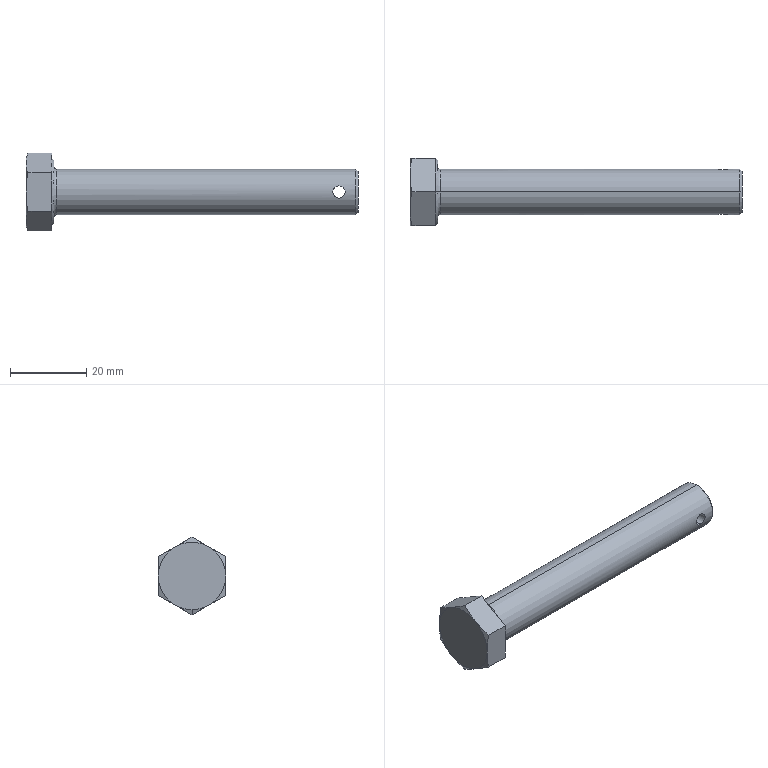Part | SolidWorks | features RevCut 3, Boss 1, Chamfer 1, Cut 1, Extrusion 1, Fillet 1, LPattern 1 | 1 solid | 32 faces | box 87.32 x 17.73 x 20.473 mm | volume 10914 mm3 | plane 15 | cone 11 | cylinder 4 | torus 2 | commonest cylinder face diameters 3.2 x2 12 x2
STEP:
#1=CARTESIAN_POINT('',(7.92,0.,6.));
#2=VERTEX_POINT('',#1);
#3=CARTESIAN_POINT('',(7.92,0.,-6.));
#4=VERTEX_POINT('',#3);
#5=CARTESIAN_POINT('',(7.92,0.,0.));
#6=DIRECTION('',(1.,0.,0.));
#7=DIRECTION('',(0.,0.,-1.));
#8=AXIS2_PLACEMENT_3D('',#5,#6,#7);
#9=CIRCLE('',#8,6.);
#10=EDGE_CURVE('',#2,#4,#9,.T.);
#11=ORIENTED_EDGE('',*,*,#10,.F.);
#12=CARTESIAN_POINT('',(7.32,0.,6.6));
#13=VERTEX_POINT('',#12);
#14=CARTESIAN_POINT('',(7.92,0.,6.6));
#15=DIRECTION('',(0.,1.,0.));
#16=DIRECTION('',(0.,0.,1.));
#17=AXIS2_PLACEMENT_3D('',#14,#15,#16);
#18=CIRCLE('',#17,0.6);
#19=EDGE_CURVE('',#2,#13,#18,.T.);
#20=ORIENTED_EDGE('',*,*,#19,.T.);
#21=CARTESIAN_POINT('',(7.32,0.,-6.6));
#22=VERTEX_POINT('',#21);
#23=CARTESIAN_POINT('',(7.32,0.,0.));
#24=DIRECTION('',(-1.,0.,0.));
#25=DIRECTION('',(0.,0.,-1.));
#26=AXIS2_PLACEMENT_3D('',#23,#24,#25);
#27=CIRCLE('',#26,6.6);
#28=EDGE_CURVE('',#22,#13,#27,.T.);
#29=ORIENTED_EDGE('',*,*,#28,.F.);
#30=CARTESIAN_POINT('',(7.92,0.,-6.6));
#31=DIRECTION('',(0.,-1.,0.));
#32=DIRECTION('',(0.,0.,-1.));
#33=AXIS2_PLACEMENT_3D('',#30,#31,#32);
#34=CIRCLE('',#33,0.6);
#35=EDGE_CURVE('',#4,#22,#34,.T.);
#36=ORIENTED_EDGE('',*,*,#35,.F.);
#37=EDGE_LOOP('',(#11,#20,#29,#36));
#38=FACE_OUTER_BOUND('',#37,.T.);
#39=CARTESIAN_POINT('',(7.92,0.,0.));
#40=DIRECTION('',(1.,0.,0.));
#41=DIRECTION('',(0.,0.,-1.));
#42=AXIS2_PLACEMENT_3D('',#39,#40,#41);
#43=TOROIDAL_SURFACE('',#42,6.6,0.6);
#44=ADVANCED_FACE('',(#38),#43,.F.);
#45=CARTESIAN_POINT('',(82.32,-5.783,-1.6));
#46=VERTEX_POINT('',#45);
#47=CARTESIAN_POINT('',(82.32,-5.783,1.6));
#48=VERTEX_POINT('',#47);
#49=CARTESIAN_POINT('',(82.32,-5.783,-1.6));
#50=CARTESIAN_POINT('',(82.111,-5.783,-1.6));
#51=CARTESIAN_POINT('',(81.899,-5.795,-1.558));
#52=CARTESIAN_POINT('',(81.61,-5.825,-1.438));
#53=CARTESIAN_POINT('',(81.517,-5.838,-1.388));
#54=CARTESIAN_POINT('',(81.343,-5.864,-1.271));
#55=CARTESIAN_POINT('',(81.263,-5.878,-1.206));
#56=CARTESIAN_POINT('',(81.115,-5.906,-1.058));
#57=CARTESIAN_POINT('',(81.048,-5.921,-0.9764));
#58=CARTESIAN_POINT('',(80.933,-5.947,-0.8037));
#59=CARTESIAN_POINT('',(80.883,-5.958,-0.712));
#60=CARTESIAN_POINT('',(80.762,-5.989,-0.4197));
#61=CARTESIAN_POINT('',(80.72,-6.,-0.2114));
#62=CARTESIAN_POINT('',(80.72,-6.,0.1051));
#63=CARTESIAN_POINT('',(80.73,-5.997,0.2093));
#64=CARTESIAN_POINT('',(80.771,-5.987,0.415));
#65=CARTESIAN_POINT('',(80.802,-5.978,0.5171));
#66=CARTESIAN_POINT('',(80.922,-5.949,0.8065));
#67=CARTESIAN_POINT('',(81.041,-5.921,0.9841));
#68=CARTESIAN_POINT('',(81.335,-5.864,1.278));
#69=CARTESIAN_POINT('',(81.512,-5.836,1.397));
#70=CARTESIAN_POINT('',(81.801,-5.805,1.517));
#71=CARTESIAN_POINT('',(81.903,-5.797,1.548));
#72=CARTESIAN_POINT('',(82.109,-5.786,1.59));
#73=CARTESIAN_POINT('',(82.214,-5.783,1.6));
#74=CARTESIAN_POINT('',(82.32,-5.783,1.6));
#75=B_SPLINE_CURVE_WITH_KNOTS('',3,(#49,#50,#51,#52,#53,#54,#55,#56,#57,#58,#59,#60,#61,#62,#63,#64,#65,#66,#67,#68,#69,#70,#71,#72,#73,#74),.UNSPECIFIED.,.F.,.F.,(4,2,2,2,2,2,2,2,2,2,2,2,4),(0.005025,0.005653,0.005967,0.006281,0.006595,0.006909,0.007537,0.007851,0.008165,0.008793,0.009421,0.009735,0.01005),.UNSPECIFIED.);
#76=EDGE_CURVE('',#46,#48,#75,.T.);
#77=ORIENTED_EDGE('',*,*,#76,.F.);
#78=CARTESIAN_POINT('',(82.32,5.783,-1.6));
#79=VERTEX_POINT('',#78);
#80=CARTESIAN_POINT('',(82.32,-8.865,-1.6));
#81=DIRECTION('',(0.,1.,0.));
#82=VECTOR('',#81,1000.);
#83=LINE('',#80,#82);
#84=EDGE_CURVE('',#46,#79,#83,.T.);
#85=ORIENTED_EDGE('',*,*,#84,.T.);
#86=CARTESIAN_POINT('',(82.32,5.783,1.6));
#87=VERTEX_POINT('',#86);
#88=CARTESIAN_POINT('',(82.32,5.783,1.6));
#89=CARTESIAN_POINT('',(82.214,5.783,1.6));
#90=CARTESIAN_POINT('',(82.109,5.786,1.59));
#91=CARTESIAN_POINT('',(81.904,5.797,1.549));
#92=CARTESIAN_POINT('',(81.802,5.805,1.518));
#93=CARTESIAN_POINT('',(81.609,5.826,1.437));
#94=CARTESIAN_POINT('',(81.517,5.838,1.388));
#95=CARTESIAN_POINT('',(81.344,5.864,1.272));
#96=CARTESIAN_POINT('',(81.262,5.878,1.205));
#97=CARTESIAN_POINT('',(81.042,5.921,0.9842));
#98=CARTESIAN_POINT('',(80.922,5.949,0.8065));
#99=CARTESIAN_POINT('',(80.763,5.988,0.4217));
#100=CARTESIAN_POINT('',(80.72,6.,0.2105));
#101=CARTESIAN_POINT('',(80.72,6.,-0.1042));
#102=CARTESIAN_POINT('',(80.73,5.997,-0.2108));
#103=CARTESIAN_POINT('',(80.772,5.986,-0.4164));
#104=CARTESIAN_POINT('',(80.802,5.979,-0.5164));
#105=CARTESIAN_POINT('',(80.923,5.949,-0.808));
#106=CARTESIAN_POINT('',(81.041,5.921,-0.9838));
#107=CARTESIAN_POINT('',(81.263,5.878,-1.206));
#108=CARTESIAN_POINT('',(81.343,5.864,-1.272));
#109=CARTESIAN_POINT('',(81.516,5.838,-1.387));
#110=CARTESIAN_POINT('',(81.61,5.825,-1.438));
#111=CARTESIAN_POINT('',(81.803,5.805,-1.518));
#112=CARTESIAN_POINT('',(81.903,5.797,-1.548));
#113=CARTESIAN_POINT('',(82.109,5.786,-1.59));
#114=CARTESIAN_POINT('',(82.215,5.783,-1.6));
#115=CARTESIAN_POINT('',(82.32,5.783,-1.6));
#116=B_SPLINE_CURVE_WITH_KNOTS('',3,(#88,#89,#90,#91,#92,#93,#94,#95,#96,#97,#98,#99,#100,#101,#102,#103,#104,#105,#106,#107,#108,#109,#110,#111,#112,#113,#114,#115),.UNSPECIFIED.,.F.,.F.,(4,2,2,2,2,2,2,2,2,2,2,2,2,4),(0.,0.0003141,0.0006281,0.0009422,0.001256,0.001884,0.002513,0.002827,0.003141,0.003769,0.004083,0.004397,0.004711,0.005025),.UNSPECIFIED.);
#117=EDGE_CURVE('',#87,#79,#116,.T.);
#118=ORIENTED_EDGE('',*,*,#117,.F.);
#119=CARTESIAN_POINT('',(82.32,-8.865,1.6));
#120=DIRECTION('',(0.,1.,0.));
#121=VECTOR('',#120,1000.);
#122=LINE('',#119,#121);
#123=EDGE_CURVE('',#48,#87,#122,.T.);
#124=ORIENTED_EDGE('',*,*,#123,.F.);
#125=EDGE_LOOP('',(#77,#85,#118,#124));
#126=FACE_OUTER_BOUND('',#125,.T.);
#127=CARTESIAN_POINT('',(82.32,-8.865,0.));
#128=DIRECTION('',(0.,1.,0.));
#129=DIRECTION('',(0.,0.,1.));
#130=AXIS2_PLACEMENT_3D('',#127,#128,#129);
#131=CYLINDRICAL_SURFACE('',#130,1.6);
#132=ADVANCED_FACE('',(#126),#131,.F.);
#133=CARTESIAN_POINT('',(87.32,0.,-5.4));
#134=VERTEX_POINT('',#133);
#135=CARTESIAN_POINT('',(87.32,0.,5.4));
#136=VERTEX_POINT('',#135);
#137=CARTESIAN_POINT('',(87.32,0.,0.));
#138=DIRECTION('',(1.,0.,0.));
#139=DIRECTION('',(0.,0.,-1.));
#140=AXIS2_PLACEMENT_3D('',#137,#138,#139);
#141=CIRCLE('',#140,5.4);
#142=EDGE_CURVE('',#134,#136,#141,.T.);
#143=ORIENTED_EDGE('',*,*,#142,.F.);
#144=CARTESIAN_POINT('',(86.72,0.,-6.));
#145=VERTEX_POINT('',#144);
#146=CARTESIAN_POINT('',(87.32,0.,-5.4));
#147=DIRECTION('',(-0.7071,0.,-0.7071));
#148=VECTOR('',#147,1000.);
#149=LINE('',#146,#148);
#150=EDGE_CURVE('',#134,#145,#149,.T.);
#151=ORIENTED_EDGE('',*,*,#150,.T.);
#152=CARTESIAN_POINT('',(86.72,0.,6.));
#153=VERTEX_POINT('',#152);
#154=CARTESIAN_POINT('',(86.72,0.,0.));
#155=DIRECTION('',(-1.,0.,0.));
#156=DIRECTION('',(0.,0.,-1.));
#157=AXIS2_PLACEMENT_3D('',#154,#155,#156);
#158=CIRCLE('',#157,6.);
#159=EDGE_CURVE('',#153,#145,#158,.T.);
#160=ORIENTED_EDGE('',*,*,#159,.F.);
#161=CARTESIAN_POINT('',(87.32,0.,5.4));
#162=DIRECTION('',(-0.7071,0.,0.7071));
#163=VECTOR('',#162,1000.);
#164=LINE('',#161,#163);
#165=EDGE_CURVE('',#136,#153,#164,.T.);
#166=ORIENTED_EDGE('',*,*,#165,.F.);
#167=EDGE_LOOP('',(#143,#151,#160,#166));
#168=FACE_OUTER_BOUND('',#167,.T.);
#169=CARTESIAN_POINT('',(87.32,0.,0.));
#170=DIRECTION('',(-1.,0.,0.));
#171=DIRECTION('',(0.,0.,1.));
#172=AXIS2_PLACEMENT_3D('',#169,#170,#171);
#173=CONICAL_SURFACE('',#172,5.4,0.7854);
#174=ADVANCED_FACE('',(#168),#173,.T.);
#175=ORIENTED_EDGE('',*,*,#117,.T.);
#176=CARTESIAN_POINT('',(82.32,5.783,-1.6));
#177=CARTESIAN_POINT('',(82.529,5.783,-1.6));
#178=CARTESIAN_POINT('',(82.741,5.795,-1.558));
#179=CARTESIAN_POINT('',(83.03,5.825,-1.438));
#180=CARTESIAN_POINT('',(83.123,5.838,-1.388));
#181=CARTESIAN_POINT('',(83.297,5.864,-1.271));
#182=CARTESIAN_POINT('',(83.377,5.878,-1.206));
#183=CARTESIAN_POINT('',(83.525,5.906,-1.058));
#184=CARTESIAN_POINT('',(83.592,5.921,-0.9764));
#185=CARTESIAN_POINT('',(83.707,5.947,-0.8037));
#186=CARTESIAN_POINT('',(83.757,5.958,-0.712));
#187=CARTESIAN_POINT('',(83.878,5.989,-0.4197));
#188=CARTESIAN_POINT('',(83.92,6.,-0.2114));
#189=CARTESIAN_POINT('',(83.92,6.,0.1051));
#190=CARTESIAN_POINT('',(83.91,5.997,0.2093));
#191=CARTESIAN_POINT('',(83.869,5.987,0.415));
#192=CARTESIAN_POINT('',(83.838,5.978,0.5171));
#193=CARTESIAN_POINT('',(83.718,5.949,0.8065));
#194=CARTESIAN_POINT('',(83.599,5.921,0.9841));
#195=CARTESIAN_POINT('',(83.305,5.864,1.278));
#196=CARTESIAN_POINT('',(83.128,5.836,1.397));
#197=CARTESIAN_POINT('',(82.839,5.805,1.517));
#198=CARTESIAN_POINT('',(82.737,5.797,1.548));
#199=CARTESIAN_POINT('',(82.531,5.786,1.59));
#200=CARTESIAN_POINT('',(82.426,5.783,1.6));
#201=CARTESIAN_POINT('',(82.32,5.783,1.6));
#202=B_SPLINE_CURVE_WITH_KNOTS('',3,(#176,#177,#178,#179,#180,#181,#182,#183,#184,#185,#186,#187,#188,#189,#190,#191,#192,#193,#194,#195,#196,#197,#198,#199,#200,#201),.UNSPECIFIED.,.F.,.F.,(4,2,2,2,2,2,2,2,2,2,2,2,4),(0.005025,0.005653,0.005967,0.006281,0.006595,0.006909,0.007537,0.007851,0.008165,0.008793,0.009421,0.009735,0.01005),.UNSPECIFIED.);
#203=EDGE_CURVE('',#79,#87,#202,.T.);
#204=ORIENTED_EDGE('',*,*,#203,.T.);
#205=EDGE_LOOP('',(#175,#204));
#206=FACE_BOUND('',#205,.T.);
#207=ORIENTED_EDGE('',*,*,#159,.T.);
#208=CARTESIAN_POINT('',(87.32,0.,-6.));
#209=DIRECTION('',(-1.,0.,0.));
#210=VECTOR('',#209,1000.);
#211=LINE('',#208,#210);
#212=EDGE_CURVE('',#145,#4,#211,.T.);
#213=ORIENTED_EDGE('',*,*,#212,.T.);
#214=CARTESIAN_POINT('',(7.92,0.,0.));
#215=DIRECTION('',(1.,0.,0.));
#216=DIRECTION('',(0.,0.,-1.));
#217=AXIS2_PLACEMENT_3D('',#214,#215,#216);
#218=CIRCLE('',#217,6.);
#219=EDGE_CURVE('',#4,#2,#218,.T.);
#220=ORIENTED_EDGE('',*,*,#219,.T.);
#221=CARTESIAN_POINT('',(87.32,0.,6.));
#222=DIRECTION('',(-1.,0.,0.));
#223=VECTOR('',#222,1000.);
#224=LINE('',#221,#223);
#225=EDGE_CURVE('',#153,#2,#224,.T.);
#226=ORIENTED_EDGE('',*,*,#225,.F.);
#227=EDGE_LOOP('',(#207,#213,#220,#226));
#228=FACE_OUTER_BOUND('',#227,.T.);
#229=CARTESIAN_POINT('',(87.32,0.,0.));
#230=DIRECTION('',(-1.,0.,0.));
#231=DIRECTION('',(0.,0.,1.));
#232=AXIS2_PLACEMENT_3D('',#229,#230,#231);
#233=CYLINDRICAL_SURFACE('',#232,6.);
#234=ADVANCED_FACE('',(#206,#228),#233,.T.);
#235=CARTESIAN_POINT('',(0.,-4.432,-7.677));
#236=VERTEX_POINT('',#235);
#237=CARTESIAN_POINT('',(0.,0.,-8.865));
#238=VERTEX_POINT('',#237);
#239=CARTESIAN_POINT('',(0.,0.,0.));
#240=DIRECTION('',(1.,0.,0.));
#241=DIRECTION('',(0.,0.,-1.));
#242=AXIS2_PLACEMENT_3D('',#239,#240,#241);
#243=CIRCLE('',#242,8.865);
#244=EDGE_CURVE('',#236,#238,#243,.T.);
#245=ORIENTED_EDGE('',*,*,#244,.T.);
#246=CARTESIAN_POINT('',(0.4992,0.,-10.236));
#247=VERTEX_POINT('',#246);
#248=CARTESIAN_POINT('',(0.,0.,-8.865));
#249=DIRECTION('',(0.342,0.,-0.9397));
#250=VECTOR('',#249,1000.);
#251=LINE('',#248,#250);
#252=EDGE_CURVE('',#238,#247,#251,.T.);
#253=ORIENTED_EDGE('',*,*,#252,.T.);
#254=CARTESIAN_POINT('',(0.4992,0.,-10.236));
#255=CARTESIAN_POINT('',(0.3439,-0.7387,-9.81));
#256=CARTESIAN_POINT('',(0.2179,-1.477,-9.383));
#257=CARTESIAN_POINT('',(0.04564,-2.955,-8.53));
#258=CARTESIAN_POINT('',(0.,-3.694,-8.104));
#259=CARTESIAN_POINT('',(0.,-4.432,-7.677));
#260=B_SPLINE_CURVE_WITH_KNOTS('',3,(#254,#255,#256,#257,#258,#259),.UNSPECIFIED.,.F.,.F.,(4,2,4),(0.000000231,0.002559,0.005118),.UNSPECIFIED.);
#261=EDGE_CURVE('',#247,#236,#260,.T.);
#262=ORIENTED_EDGE('',*,*,#261,.T.);
#263=EDGE_LOOP('',(#245,#253,#262));
#264=FACE_OUTER_BOUND('',#263,.T.);
#265=CARTESIAN_POINT('',(0.,0.,0.));
#266=DIRECTION('',(1.,0.,0.));
#267=DIRECTION('',(0.,0.,-1.));
#268=AXIS2_PLACEMENT_3D('',#265,#266,#267);
#269=CONICAL_SURFACE('',#268,8.865,1.222);
#270=ADVANCED_FACE('',(#264),#269,.T.);
#271=CARTESIAN_POINT('',(7.32,0.,8.315));
#272=VERTEX_POINT('',#271);
#273=CARTESIAN_POINT('',(7.32,0.,-8.315));
#274=VERTEX_POINT('',#273);
#275=CARTESIAN_POINT('',(7.32,0.,0.));
#276=DIRECTION('',(-1.,0.,0.));
#277=DIRECTION('',(0.,0.,1.));
#278=AXIS2_PLACEMENT_3D('',#275,#276,#277);
#279=CIRCLE('',#278,8.315);
#280=EDGE_CURVE('',#272,#274,#279,.T.);
#281=ORIENTED_EDGE('',*,*,#280,.T.);
#282=CARTESIAN_POINT('',(6.72,0.,-8.915));
#283=VERTEX_POINT('',#282);
#284=CARTESIAN_POINT('',(6.72,0.,-8.915));
#285=DIRECTION('',(-0.7071,0.,-0.7071));
#286=VECTOR('',#285,1000.);
#287=LINE('',#284,#286);
#288=EDGE_CURVE('',#274,#283,#287,.T.);
#289=ORIENTED_EDGE('',*,*,#288,.T.);
#290=CARTESIAN_POINT('',(6.72,3.616,-8.149));
#291=VERTEX_POINT('',#290);
#292=CARTESIAN_POINT('',(6.72,0.,0.));
#293=DIRECTION('',(-1.,0.,0.));
#294=DIRECTION('',(0.,0.,1.));
#295=AXIS2_PLACEMENT_3D('',#292,#293,#294);
#296=CIRCLE('',#295,8.915);
#297=EDGE_CURVE('',#291,#283,#296,.T.);
#298=ORIENTED_EDGE('',*,*,#297,.F.);
#299=CARTESIAN_POINT('',(6.72,5.249,-7.206));
#300=VERTEX_POINT('',#299);
#301=CARTESIAN_POINT('',(6.72,3.616,-8.149));
#302=CARTESIAN_POINT('',(6.786,4.16,-7.834));
#303=CARTESIAN_POINT('',(6.786,4.705,-7.52));
#304=CARTESIAN_POINT('',(6.72,5.249,-7.206));
#305=B_SPLINE_CURVE_WITH_KNOTS('',3,(#301,#302,#303,#304),.UNSPECIFIED.,.F.,.F.,(4,4),(0.000001889,0.001888),.UNSPECIFIED.);
#306=EDGE_CURVE('',#291,#300,#305,.T.);
#307=ORIENTED_EDGE('',*,*,#306,.T.);
#308=CARTESIAN_POINT('',(6.72,8.865,-0.9429));
#309=VERTEX_POINT('',#308);
#310=CARTESIAN_POINT('',(6.72,0.,0.));
#311=DIRECTION('',(-1.,0.,0.));
#312=DIRECTION('',(0.,0.,1.));
#313=AXIS2_PLACEMENT_3D('',#310,#311,#312);
#314=CIRCLE('',#313,8.915);
#315=EDGE_CURVE('',#309,#300,#314,.T.);
#316=ORIENTED_EDGE('',*,*,#315,.F.);
#317=CARTESIAN_POINT('',(6.72,8.865,0.9429));
#318=VERTEX_POINT('',#317);
#319=CARTESIAN_POINT('',(6.72,8.865,-0.9429));
#320=CARTESIAN_POINT('',(6.787,8.865,-0.3136));
#321=CARTESIAN_POINT('',(6.786,8.865,0.315));
#322=CARTESIAN_POINT('',(6.72,8.865,0.9429));
#323=B_SPLINE_CURVE_WITH_KNOTS('',3,(#319,#320,#321,#322),.UNSPECIFIED.,.F.,.F.,(4,4),(0.004033,0.005912),.UNSPECIFIED.);
#324=EDGE_CURVE('',#309,#318,#323,.T.);
#325=ORIENTED_EDGE('',*,*,#324,.T.);
#326=CARTESIAN_POINT('',(6.72,5.249,7.206));
#327=VERTEX_POINT('',#326);
#328=CARTESIAN_POINT('',(6.72,0.,0.));
#329=DIRECTION('',(-1.,0.,0.));
#330=DIRECTION('',(0.,0.,1.));
#331=AXIS2_PLACEMENT_3D('',#328,#329,#330);
#332=CIRCLE('',#331,8.915);
#333=EDGE_CURVE('',#327,#318,#332,.T.);
#334=ORIENTED_EDGE('',*,*,#333,.F.);
#335=CARTESIAN_POINT('',(6.72,3.616,8.149));
#336=VERTEX_POINT('',#335);
#337=CARTESIAN_POINT('',(6.72,5.249,7.206));
#338=CARTESIAN_POINT('',(6.786,4.705,7.52));
#339=CARTESIAN_POINT('',(6.786,4.16,7.834));
#340=CARTESIAN_POINT('',(6.72,3.616,8.149));
#341=B_SPLINE_CURVE_WITH_KNOTS('',3,(#337,#338,#339,#340),.UNSPECIFIED.,.F.,.F.,(4,4),(0.000001889,0.001888),.UNSPECIFIED.);
#342=EDGE_CURVE('',#327,#336,#341,.T.);
#343=ORIENTED_EDGE('',*,*,#342,.T.);
#344=CARTESIAN_POINT('',(6.72,0.,8.915));
#345=VERTEX_POINT('',#344);
#346=CARTESIAN_POINT('',(6.72,0.,0.));
#347=DIRECTION('',(-1.,0.,0.));
#348=DIRECTION('',(0.,0.,1.));
#349=AXIS2_PLACEMENT_3D('',#346,#347,#348);
#350=CIRCLE('',#349,8.915);
#351=EDGE_CURVE('',#345,#336,#350,.T.);
#352=ORIENTED_EDGE('',*,*,#351,.F.);
#353=CARTESIAN_POINT('',(6.72,0.,8.915));
#354=DIRECTION('',(-0.7071,0.,0.7071));
#355=VECTOR('',#354,1000.);
#356=LINE('',#353,#355);
#357=EDGE_CURVE('',#272,#345,#356,.T.);
#358=ORIENTED_EDGE('',*,*,#357,.F.);
#359=EDGE_LOOP('',(#281,#289,#298,#307,#316,#325,#334,#343,#352,#358));
#360=FACE_OUTER_BOUND('',#359,.T.);
#361=CARTESIAN_POINT('',(6.72,0.,0.));
#362=DIRECTION('',(-1.,0.,0.));
#363=DIRECTION('',(0.,0.,1.));
#364=AXIS2_PLACEMENT_3D('',#361,#362,#363);
#365=CONICAL_SURFACE('',#364,8.915,0.7854);
#366=ADVANCED_FACE('',(#360),#365,.T.);
#367=ORIENTED_EDGE('',*,*,#28,.T.);
#368=CARTESIAN_POINT('',(7.32,0.,0.));
#369=DIRECTION('',(-1.,0.,0.));
#370=DIRECTION('',(0.,0.,-1.));
#371=AXIS2_PLACEMENT_3D('',#368,#369,#370);
#372=CIRCLE('',#371,6.6);
#373=EDGE_CURVE('',#13,#22,#372,.T.);
#374=ORIENTED_EDGE('',*,*,#373,.T.);
#375=EDGE_LOOP('',(#367,#374));
#376=FACE_BOUND('',#375,.T.);
#377=ORIENTED_EDGE('',*,*,#280,.F.);
#378=CARTESIAN_POINT('',(7.32,0.,0.));
#379=DIRECTION('',(-1.,0.,0.));
#380=DIRECTION('',(0.,0.,1.));
#381=AXIS2_PLACEMENT_3D('',#378,#379,#380);
#382=CIRCLE('',#381,8.315);
#383=EDGE_CURVE('',#274,#272,#382,.T.);
#384=ORIENTED_EDGE('',*,*,#383,.F.);
#385=EDGE_LOOP('',(#377,#384));
#386=FACE_OUTER_BOUND('',#385,.T.);
#387=CARTESIAN_POINT('',(7.32,0.,-10.236));
#388=DIRECTION('',(1.,0.,0.));
#389=DIRECTION('',(0.,0.,-1.));
#390=AXIS2_PLACEMENT_3D('',#387,#388,#389);
#391=PLANE('',#390);
#392=ADVANCED_FACE('',(#376,#386),#391,.T.);
#393=ORIENTED_EDGE('',*,*,#261,.F.);
#394=CARTESIAN_POINT('',(6.72,0.,-10.236));
#395=VERTEX_POINT('',#394);
#396=CARTESIAN_POINT('',(7.32,0.,-10.236));
#397=DIRECTION('',(-1.,0.,0.));
#398=VECTOR('',#397,1000.);
#399=LINE('',#396,#398);
#400=EDGE_CURVE('',#395,#247,#399,.T.);
#401=ORIENTED_EDGE('',*,*,#400,.F.);
#402=CARTESIAN_POINT('',(6.72,-3.616,-8.149));
#403=VERTEX_POINT('',#402);
#404=CARTESIAN_POINT('',(6.72,-8.865,-5.118));
#405=DIRECTION('',(0.,0.866,-0.5));
#406=VECTOR('',#405,1000.);
#407=LINE('',#404,#406);
#408=EDGE_CURVE('',#403,#395,#407,.T.);
#409=ORIENTED_EDGE('',*,*,#408,.F.);
#410=CARTESIAN_POINT('',(6.72,-5.249,-7.206));
#411=VERTEX_POINT('',#410);
#412=CARTESIAN_POINT('',(6.72,-5.249,-7.206));
#413=CARTESIAN_POINT('',(6.786,-4.705,-7.52));
#414=CARTESIAN_POINT('',(6.786,-4.16,-7.834));
#415=CARTESIAN_POINT('',(6.72,-3.616,-8.149));
#416=B_SPLINE_CURVE_WITH_KNOTS('',3,(#412,#413,#414,#415),.UNSPECIFIED.,.F.,.F.,(4,4),(0.000001889,0.001888),.UNSPECIFIED.);
#417=EDGE_CURVE('',#411,#403,#416,.T.);
#418=ORIENTED_EDGE('',*,*,#417,.F.);
#419=CARTESIAN_POINT('',(6.72,-8.865,-5.118));
#420=VERTEX_POINT('',#419);
#421=CARTESIAN_POINT('',(6.72,-8.865,-5.118));
#422=DIRECTION('',(0.,0.866,-0.5));
#423=VECTOR('',#422,1000.);
#424=LINE('',#421,#423);
#425=EDGE_CURVE('',#420,#411,#424,.T.);
#426=ORIENTED_EDGE('',*,*,#425,.F.);
#427=CARTESIAN_POINT('',(0.4992,-8.865,-5.118));
#428=VERTEX_POINT('',#427);
#429=CARTESIAN_POINT('',(7.32,-8.865,-5.118));
#430=DIRECTION('',(-1.,0.,0.));
#431=VECTOR('',#430,1000.);
#432=LINE('',#429,#431);
#433=EDGE_CURVE('',#420,#428,#432,.T.);
#434=ORIENTED_EDGE('',*,*,#433,.T.);
#435=CARTESIAN_POINT('',(0.,-4.432,-7.677));
#436=CARTESIAN_POINT('',(0.,-5.171,-7.251));
#437=CARTESIAN_POINT('',(0.04564,-5.91,-6.824));
#438=CARTESIAN_POINT('',(0.2179,-7.387,-5.971));
#439=CARTESIAN_POINT('',(0.3439,-8.126,-5.545));
#440=CARTESIAN_POINT('',(0.4992,-8.865,-5.118));
#441=B_SPLINE_CURVE_WITH_KNOTS('',3,(#435,#436,#437,#438,#439,#440),.UNSPECIFIED.,.F.,.F.,(4,2,4),(0.005118,0.007678,0.01024),.UNSPECIFIED.);
#442=EDGE_CURVE('',#236,#428,#441,.T.);
#443=ORIENTED_EDGE('',*,*,#442,.F.);
#444=EDGE_LOOP('',(#393,#401,#409,#418,#426,#434,#443));
#445=FACE_OUTER_BOUND('',#444,.T.);
#446=CARTESIAN_POINT('',(7.32,-8.865,-5.118));
#447=DIRECTION('',(0.,0.5,0.866));
#448=DIRECTION('',(0.,-0.866,0.5));
#449=AXIS2_PLACEMENT_3D('',#446,#447,#448);
#450=PLANE('',#449);
#451=ADVANCED_FACE('',(#445),#450,.F.);
#452=CARTESIAN_POINT('',(0.4992,8.865,-5.118));
#453=VERTEX_POINT('',#452);
#454=CARTESIAN_POINT('',(0.,4.433,-7.677));
#455=VERTEX_POINT('',#454);
#456=CARTESIAN_POINT('',(0.4992,8.865,-5.118));
#457=CARTESIAN_POINT('',(0.3439,8.126,-5.545));
#458=CARTESIAN_POINT('',(0.2179,7.388,-5.971));
#459=CARTESIAN_POINT('',(0.04564,5.91,-6.824));
#460=CARTESIAN_POINT('',(0.,5.171,-7.251));
#461=CARTESIAN_POINT('',(0.,4.433,-7.677));
#462=B_SPLINE_CURVE_WITH_KNOTS('',3,(#456,#457,#458,#459,#460,#461),.UNSPECIFIED.,.F.,.F.,(4,2,4),(0.000000231,0.002559,0.005118),.UNSPECIFIED.);
#463=EDGE_CURVE('',#453,#455,#462,.T.);
#464=ORIENTED_EDGE('',*,*,#463,.F.);
#465=CARTESIAN_POINT('',(6.72,8.865,-5.118));
#466=VERTEX_POINT('',#465);
#467=CARTESIAN_POINT('',(7.32,8.865,-5.118));
#468=DIRECTION('',(-1.,0.,0.));
#469=VECTOR('',#468,1000.);
#470=LINE('',#467,#469);
#471=EDGE_CURVE('',#466,#453,#470,.T.);
#472=ORIENTED_EDGE('',*,*,#471,.F.);
#473=CARTESIAN_POINT('',(6.72,0.,-10.236));
#474=DIRECTION('',(0.,0.866,0.5));
#475=VECTOR('',#474,1000.);
#476=LINE('',#473,#475);
#477=EDGE_CURVE('',#300,#466,#476,.T.);
#478=ORIENTED_EDGE('',*,*,#477,.F.);
#479=ORIENTED_EDGE('',*,*,#306,.F.);
#480=CARTESIAN_POINT('',(6.72,0.,-10.236));
#481=DIRECTION('',(0.,0.866,0.5));
#482=VECTOR('',#481,1000.);
#483=LINE('',#480,#482);
#484=EDGE_CURVE('',#395,#291,#483,.T.);
#485=ORIENTED_EDGE('',*,*,#484,.F.);
#486=ORIENTED_EDGE('',*,*,#400,.T.);
#487=CARTESIAN_POINT('',(0.,4.433,-7.677));
#488=CARTESIAN_POINT('',(0.,3.694,-8.104));
#489=CARTESIAN_POINT('',(0.04564,2.955,-8.53));
#490=CARTESIAN_POINT('',(0.2179,1.478,-9.383));
#491=CARTESIAN_POINT('',(0.3439,0.7388,-9.81));
#492=CARTESIAN_POINT('',(0.4992,0.,-10.236));
#493=B_SPLINE_CURVE_WITH_KNOTS('',3,(#487,#488,#489,#490,#491,#492),.UNSPECIFIED.,.F.,.F.,(4,2,4),(0.005118,0.007678,0.01024),.UNSPECIFIED.);
#494=EDGE_CURVE('',#455,#247,#493,.T.);
#495=ORIENTED_EDGE('',*,*,#494,.F.);
#496=EDGE_LOOP('',(#464,#472,#478,#479,#485,#486,#495));
#497=FACE_OUTER_BOUND('',#496,.T.);
#498=CARTESIAN_POINT('',(7.32,0.,-10.236));
#499=DIRECTION('',(0.,-0.5,0.866));
#500=DIRECTION('',(0.,-0.866,-0.5));
#501=AXIS2_PLACEMENT_3D('',#498,#499,#500);
#502=PLANE('',#501);
#503=ADVANCED_FACE('',(#497),#502,.F.);
#504=CARTESIAN_POINT('',(0.4992,8.865,5.118));
#505=VERTEX_POINT('',#504);
#506=CARTESIAN_POINT('',(0.,8.865,0.));
#507=VERTEX_POINT('',#506);
#508=CARTESIAN_POINT('',(0.4992,8.865,5.118));
#509=CARTESIAN_POINT('',(0.3443,8.865,4.267));
#510=CARTESIAN_POINT('',(0.2182,8.865,3.415));
#511=CARTESIAN_POINT('',(0.04582,8.865,1.709));
#512=CARTESIAN_POINT('',(0.,8.865,0.8548));
#513=CARTESIAN_POINT('',(0.,8.865,0.));
#514=B_SPLINE_CURVE_WITH_KNOTS('',3,(#508,#509,#510,#511,#512,#513),.UNSPECIFIED.,.F.,.F.,(4,2,4),(0.01846,0.02104,0.02362),.UNSPECIFIED.);
#515=EDGE_CURVE('',#505,#507,#514,.T.);
#516=ORIENTED_EDGE('',*,*,#515,.F.);
#517=CARTESIAN_POINT('',(6.72,8.865,5.118));
#518=VERTEX_POINT('',#517);
#519=CARTESIAN_POINT('',(7.32,8.865,5.118));
#520=DIRECTION('',(-1.,0.,0.));
#521=VECTOR('',#520,1000.);
#522=LINE('',#519,#521);
#523=EDGE_CURVE('',#518,#505,#522,.T.);
#524=ORIENTED_EDGE('',*,*,#523,.F.);
#525=CARTESIAN_POINT('',(6.72,8.865,-5.118));
#526=DIRECTION('',(0.,0.,1.));
#527=VECTOR('',#526,1000.);
#528=LINE('',#525,#527);
#529=EDGE_CURVE('',#318,#518,#528,.T.);
#530=ORIENTED_EDGE('',*,*,#529,.F.);
#531=ORIENTED_EDGE('',*,*,#324,.F.);
#532=CARTESIAN_POINT('',(6.72,8.865,-5.118));
#533=DIRECTION('',(0.,0.,1.));
#534=VECTOR('',#533,1000.);
#535=LINE('',#532,#534);
#536=EDGE_CURVE('',#466,#309,#535,.T.);
#537=ORIENTED_EDGE('',*,*,#536,.F.);
#538=ORIENTED_EDGE('',*,*,#471,.T.);
#539=CARTESIAN_POINT('',(0.,8.865,0.));
#540=CARTESIAN_POINT('',(0.,8.865,-0.8523));
#541=CARTESIAN_POINT('',(0.04558,8.865,-1.706));
#542=CARTESIAN_POINT('',(0.2181,8.865,-3.414));
#543=CARTESIAN_POINT('',(0.3449,8.865,-4.271));
#544=CARTESIAN_POINT('',(0.4992,8.865,-5.118));
#545=B_SPLINE_CURVE_WITH_KNOTS('',3,(#539,#540,#541,#542,#543,#544),.UNSPECIFIED.,.F.,.F.,(4,2,4),(0.02362,0.02619,0.02876),.UNSPECIFIED.);
#546=EDGE_CURVE('',#507,#453,#545,.T.);
#547=ORIENTED_EDGE('',*,*,#546,.F.);
#548=EDGE_LOOP('',(#516,#524,#530,#531,#537,#538,#547));
#549=FACE_OUTER_BOUND('',#548,.T.);
#550=CARTESIAN_POINT('',(7.32,8.865,-5.118));
#551=DIRECTION('',(0.,-1.,0.));
#552=DIRECTION('',(0.,0.,-1.));
#553=AXIS2_PLACEMENT_3D('',#550,#551,#552);
#554=PLANE('',#553);
#555=ADVANCED_FACE('',(#549),#554,.F.);
#556=CARTESIAN_POINT('',(0.4992,0.,10.236));
#557=VERTEX_POINT('',#556);
#558=CARTESIAN_POINT('',(0.,4.432,7.677));
#559=VERTEX_POINT('',#558);
#560=CARTESIAN_POINT('',(0.4992,0.,10.236));
#561=CARTESIAN_POINT('',(0.3439,0.7387,9.81));
#562=CARTESIAN_POINT('',(0.2179,1.477,9.383));
#563=CARTESIAN_POINT('',(0.04564,2.955,8.53));
#564=CARTESIAN_POINT('',(0.,3.694,8.104));
#565=CARTESIAN_POINT('',(0.,4.432,7.677));
#566=B_SPLINE_CURVE_WITH_KNOTS('',3,(#560,#561,#562,#563,#564,#565),.UNSPECIFIED.,.F.,.F.,(4,2,4),(0.000000231,0.002559,0.005118),.UNSPECIFIED.);
#567=EDGE_CURVE('',#557,#559,#566,.T.);
#568=ORIENTED_EDGE('',*,*,#567,.F.);
#569=CARTESIAN_POINT('',(6.72,0.,10.236));
#570=VERTEX_POINT('',#569);
#571=CARTESIAN_POINT('',(7.32,0.,10.236));
#572=DIRECTION('',(-1.,0.,0.));
#573=VECTOR('',#572,1000.);
#574=LINE('',#571,#573);
#575=EDGE_CURVE('',#570,#557,#574,.T.);
#576=ORIENTED_EDGE('',*,*,#575,.F.);
#577=CARTESIAN_POINT('',(6.72,8.865,5.118));
#578=DIRECTION('',(0.,-0.866,0.5));
#579=VECTOR('',#578,1000.);
#580=LINE('',#577,#579);
#581=EDGE_CURVE('',#336,#570,#580,.T.);
#582=ORIENTED_EDGE('',*,*,#581,.F.);
#583=ORIENTED_EDGE('',*,*,#342,.F.);
#584=CARTESIAN_POINT('',(6.72,8.865,5.118));
#585=DIRECTION('',(0.,-0.866,0.5));
#586=VECTOR('',#585,1000.);
#587=LINE('',#584,#586);
#588=EDGE_CURVE('',#518,#327,#587,.T.);
#589=ORIENTED_EDGE('',*,*,#588,.F.);
#590=ORIENTED_EDGE('',*,*,#523,.T.);
#591=CARTESIAN_POINT('',(0.,4.432,7.677));
#592=CARTESIAN_POINT('',(0.,5.171,7.251));
#593=CARTESIAN_POINT('',(0.04564,5.91,6.824));
#594=CARTESIAN_POINT('',(0.2179,7.387,5.971));
#595=CARTESIAN_POINT('',(0.3439,8.126,5.545));
#596=CARTESIAN_POINT('',(0.4992,8.865,5.118));
#597=B_SPLINE_CURVE_WITH_KNOTS('',3,(#591,#592,#593,#594,#595,#596),.UNSPECIFIED.,.F.,.F.,(4,2,4),(0.005118,0.007678,0.01024),.UNSPECIFIED.);
#598=EDGE_CURVE('',#559,#505,#597,.T.);
#599=ORIENTED_EDGE('',*,*,#598,.F.);
#600=EDGE_LOOP('',(#568,#576,#582,#583,#589,#590,#599));
#601=FACE_OUTER_BOUND('',#600,.T.);
#602=CARTESIAN_POINT('',(7.32,8.865,5.118));
#603=DIRECTION('',(0.,-0.5,-0.866));
#604=DIRECTION('',(0.,0.866,-0.5));
#605=AXIS2_PLACEMENT_3D('',#602,#603,#604);
#606=PLANE('',#605);
#607=ADVANCED_FACE('',(#601),#606,.F.);
#608=CARTESIAN_POINT('',(0.4992,-8.865,5.118));
#609=VERTEX_POINT('',#608);
#610=CARTESIAN_POINT('',(0.,-4.433,7.677));
#611=VERTEX_POINT('',#610);
#612=CARTESIAN_POINT('',(0.4992,-8.865,5.118));
#613=CARTESIAN_POINT('',(0.3439,-8.126,5.545));
#614=CARTESIAN_POINT('',(0.2179,-7.387,5.971));
#615=CARTESIAN_POINT('',(0.04564,-5.91,6.824));
#616=CARTESIAN_POINT('',(0.,-5.171,7.251));
#617=CARTESIAN_POINT('',(0.,-4.433,7.677));
#618=B_SPLINE_CURVE_WITH_KNOTS('',3,(#612,#613,#614,#615,#616,#617),.UNSPECIFIED.,.F.,.F.,(4,2,4),(0.000000231,0.002559,0.005118),.UNSPECIFIED.);
#619=EDGE_CURVE('',#609,#611,#618,.T.);
#620=ORIENTED_EDGE('',*,*,#619,.F.);
#621=CARTESIAN_POINT('',(6.72,-8.865,5.118));
#622=VERTEX_POINT('',#621);
#623=CARTESIAN_POINT('',(7.32,-8.865,5.118));
#624=DIRECTION('',(-1.,0.,0.));
#625=VECTOR('',#624,1000.);
#626=LINE('',#623,#625);
#627=EDGE_CURVE('',#622,#609,#626,.T.);
#628=ORIENTED_EDGE('',*,*,#627,.F.);
#629=CARTESIAN_POINT('',(6.72,-5.249,7.206));
#630=VERTEX_POINT('',#629);
#631=CARTESIAN_POINT('',(6.72,0.,10.236));
#632=DIRECTION('',(0.,-0.866,-0.5));
#633=VECTOR('',#632,1000.);
#634=LINE('',#631,#633);
#635=EDGE_CURVE('',#630,#622,#634,.T.);
#636=ORIENTED_EDGE('',*,*,#635,.F.);
#637=CARTESIAN_POINT('',(6.72,-3.616,8.149));
#638=VERTEX_POINT('',#637);
#639=CARTESIAN_POINT('',(6.72,-3.616,8.149));
#640=CARTESIAN_POINT('',(6.786,-4.16,7.834));
#641=CARTESIAN_POINT('',(6.786,-4.705,7.52));
#642=CARTESIAN_POINT('',(6.72,-5.249,7.206));
#643=B_SPLINE_CURVE_WITH_KNOTS('',3,(#639,#640,#641,#642),.UNSPECIFIED.,.F.,.F.,(4,4),(0.000001889,0.001888),.UNSPECIFIED.);
#644=EDGE_CURVE('',#638,#630,#643,.T.);
#645=ORIENTED_EDGE('',*,*,#644,.F.);
#646=CARTESIAN_POINT('',(6.72,0.,10.236));
#647=DIRECTION('',(0.,-0.866,-0.5));
#648=VECTOR('',#647,1000.);
#649=LINE('',#646,#648);
#650=EDGE_CURVE('',#570,#638,#649,.T.);
#651=ORIENTED_EDGE('',*,*,#650,.F.);
#652=ORIENTED_EDGE('',*,*,#575,.T.);
#653=CARTESIAN_POINT('',(0.,-4.433,7.677));
#654=CARTESIAN_POINT('',(0.,-3.694,8.104));
#655=CARTESIAN_POINT('',(0.04564,-2.955,8.53));
#656=CARTESIAN_POINT('',(0.2179,-1.477,9.383));
#657=CARTESIAN_POINT('',(0.3439,-0.7387,9.81));
#658=CARTESIAN_POINT('',(0.4992,0.,10.236));
#659=B_SPLINE_CURVE_WITH_KNOTS('',3,(#653,#654,#655,#656,#657,#658),.UNSPECIFIED.,.F.,.F.,(4,2,4),(0.005118,0.007678,0.01024),.UNSPECIFIED.);
#660=EDGE_CURVE('',#611,#557,#659,.T.);
#661=ORIENTED_EDGE('',*,*,#660,.F.);
#662=EDGE_LOOP('',(#620,#628,#636,#645,#651,#652,#661));
#663=FACE_OUTER_BOUND('',#662,.T.);
#664=CARTESIAN_POINT('',(7.32,0.,10.236));
#665=DIRECTION('',(0.,0.5,-0.866));
#666=DIRECTION('',(0.,0.866,0.5));
#667=AXIS2_PLACEMENT_3D('',#664,#665,#666);
#668=PLANE('',#667);
#669=ADVANCED_FACE('',(#663),#668,.F.);
#670=CARTESIAN_POINT('',(0.,-8.865,0.));
#671=VERTEX_POINT('',#670);
#672=CARTESIAN_POINT('',(0.4992,-8.865,-5.118));
#673=CARTESIAN_POINT('',(0.3449,-8.865,-4.271));
#674=CARTESIAN_POINT('',(0.2181,-8.865,-3.414));
#675=CARTESIAN_POINT('',(0.04558,-8.865,-1.706));
#676=CARTESIAN_POINT('',(0.,-8.865,-0.8523));
#677=CARTESIAN_POINT('',(0.,-8.865,0.));
#678=B_SPLINE_CURVE_WITH_KNOTS('',3,(#672,#673,#674,#675,#676,#677),.UNSPECIFIED.,.F.,.F.,(4,2,4),(0.008707,0.01129,0.01387),.UNSPECIFIED.);
#679=EDGE_CURVE('',#428,#671,#678,.T.);
#680=ORIENTED_EDGE('',*,*,#679,.F.);
#681=ORIENTED_EDGE('',*,*,#433,.F.);
#682=CARTESIAN_POINT('',(6.72,-8.865,-0.9429));
#683=VERTEX_POINT('',#682);
#684=CARTESIAN_POINT('',(6.72,-8.865,5.118));
#685=DIRECTION('',(0.,0.,-1.));
#686=VECTOR('',#685,1000.);
#687=LINE('',#684,#686);
#688=EDGE_CURVE('',#683,#420,#687,.T.);
#689=ORIENTED_EDGE('',*,*,#688,.F.);
#690=CARTESIAN_POINT('',(6.72,-8.865,0.9429));
#691=VERTEX_POINT('',#690);
#692=CARTESIAN_POINT('',(6.72,-8.865,0.9429));
#693=CARTESIAN_POINT('',(6.786,-8.865,0.315));
#694=CARTESIAN_POINT('',(6.787,-8.865,-0.3136));
#695=CARTESIAN_POINT('',(6.72,-8.865,-0.9429));
#696=B_SPLINE_CURVE_WITH_KNOTS('',3,(#692,#693,#694,#695),.UNSPECIFIED.,.F.,.F.,(4,4),(0.004457,0.006334),.UNSPECIFIED.);
#697=EDGE_CURVE('',#691,#683,#696,.T.);
#698=ORIENTED_EDGE('',*,*,#697,.F.);
#699=CARTESIAN_POINT('',(6.72,-8.865,5.118));
#700=DIRECTION('',(0.,0.,-1.));
#701=VECTOR('',#700,1000.);
#702=LINE('',#699,#701);
#703=EDGE_CURVE('',#622,#691,#702,.T.);
#704=ORIENTED_EDGE('',*,*,#703,.F.);
#705=ORIENTED_EDGE('',*,*,#627,.T.);
#706=CARTESIAN_POINT('',(0.,-8.865,0.));
#707=CARTESIAN_POINT('',(0.,-8.865,0.8548));
#708=CARTESIAN_POINT('',(0.04582,-8.865,1.709));
#709=CARTESIAN_POINT('',(0.2182,-8.865,3.415));
#710=CARTESIAN_POINT('',(0.3443,-8.865,4.267));
#711=CARTESIAN_POINT('',(0.4992,-8.865,5.118));
#712=B_SPLINE_CURVE_WITH_KNOTS('',3,(#706,#707,#708,#709,#710,#711),.UNSPECIFIED.,.F.,.F.,(4,2,4),(0.01387,0.01645,0.01904),.UNSPECIFIED.);
#713=EDGE_CURVE('',#671,#609,#712,.T.);
#714=ORIENTED_EDGE('',*,*,#713,.F.);
#715=EDGE_LOOP('',(#680,#681,#689,#698,#704,#705,#714));
#716=FACE_OUTER_BOUND('',#715,.T.);
#717=CARTESIAN_POINT('',(7.32,-8.865,5.118));
#718=DIRECTION('',(0.,1.,0.));
#719=DIRECTION('',(0.,0.,1.));
#720=AXIS2_PLACEMENT_3D('',#717,#718,#719);
#721=PLANE('',#720);
#722=ADVANCED_FACE('',(#716),#721,.F.);
#723=ORIENTED_EDGE('',*,*,#408,.T.);
#724=ORIENTED_EDGE('',*,*,#484,.T.);
#725=ORIENTED_EDGE('',*,*,#297,.T.);
#726=CARTESIAN_POINT('',(6.72,0.,0.));
#727=DIRECTION('',(-1.,0.,0.));
#728=DIRECTION('',(0.,0.,1.));
#729=AXIS2_PLACEMENT_3D('',#726,#727,#728);
#730=CIRCLE('',#729,8.915);
#731=EDGE_CURVE('',#283,#403,#730,.T.);
#732=ORIENTED_EDGE('',*,*,#731,.T.);
#733=EDGE_LOOP('',(#723,#724,#725,#732));
#734=FACE_OUTER_BOUND('',#733,.T.);
#735=CARTESIAN_POINT('',(6.72,0.,-8.915));
#736=DIRECTION('',(1.,0.,0.));
#737=DIRECTION('',(0.,0.,-1.));
#738=AXIS2_PLACEMENT_3D('',#735,#736,#737);
#739=PLANE('',#738);
#740=ADVANCED_FACE('',(#734),#739,.T.);
#741=ORIENTED_EDGE('',*,*,#477,.T.);
#742=ORIENTED_EDGE('',*,*,#536,.T.);
#743=ORIENTED_EDGE('',*,*,#315,.T.);
#744=EDGE_LOOP('',(#741,#742,#743));
#745=FACE_OUTER_BOUND('',#744,.T.);
#746=CARTESIAN_POINT('',(6.72,0.,-8.915));
#747=DIRECTION('',(1.,0.,0.));
#748=DIRECTION('',(0.,0.,-1.));
#749=AXIS2_PLACEMENT_3D('',#746,#747,#748);
#750=PLANE('',#749);
#751=ADVANCED_FACE('',(#745),#750,.T.);
#752=ORIENTED_EDGE('',*,*,#529,.T.);
#753=ORIENTED_EDGE('',*,*,#588,.T.);
#754=ORIENTED_EDGE('',*,*,#333,.T.);
#755=EDGE_LOOP('',(#752,#753,#754));
#756=FACE_OUTER_BOUND('',#755,.T.);
#757=CARTESIAN_POINT('',(6.72,0.,-8.915));
#758=DIRECTION('',(1.,0.,0.));
#759=DIRECTION('',(0.,0.,-1.));
#760=AXIS2_PLACEMENT_3D('',#757,#758,#759);
#761=PLANE('',#760);
#762=ADVANCED_FACE('',(#756),#761,.T.);
#763=ORIENTED_EDGE('',*,*,#581,.T.);
#764=ORIENTED_EDGE('',*,*,#650,.T.);
#765=CARTESIAN_POINT('',(6.72,0.,0.));
#766=DIRECTION('',(-1.,0.,0.));
#767=DIRECTION('',(0.,0.,1.));
#768=AXIS2_PLACEMENT_3D('',#765,#766,#767);
#769=CIRCLE('',#768,8.915);
#770=EDGE_CURVE('',#638,#345,#769,.T.);
#771=ORIENTED_EDGE('',*,*,#770,.T.);
#772=ORIENTED_EDGE('',*,*,#351,.T.);
#773=EDGE_LOOP('',(#763,#764,#771,#772));
#774=FACE_OUTER_BOUND('',#773,.T.);
#775=CARTESIAN_POINT('',(6.72,0.,-8.915));
#776=DIRECTION('',(1.,0.,0.));
#777=DIRECTION('',(0.,0.,-1.));
#778=AXIS2_PLACEMENT_3D('',#775,#776,#777);
#779=PLANE('',#778);
#780=ADVANCED_FACE('',(#774),#779,.T.);
#781=ORIENTED_EDGE('',*,*,#635,.T.);
#782=ORIENTED_EDGE('',*,*,#703,.T.);
#783=CARTESIAN_POINT('',(6.72,0.,0.));
#784=DIRECTION('',(-1.,0.,0.));
#785=DIRECTION('',(0.,0.,1.));
#786=AXIS2_PLACEMENT_3D('',#783,#784,#785);
#787=CIRCLE('',#786,8.915);
#788=EDGE_CURVE('',#691,#630,#787,.T.);
#789=ORIENTED_EDGE('',*,*,#788,.T.);
#790=EDGE_LOOP('',(#781,#782,#789));
#791=FACE_OUTER_BOUND('',#790,.T.);
#792=CARTESIAN_POINT('',(6.72,0.,-8.915));
#793=DIRECTION('',(1.,0.,0.));
#794=DIRECTION('',(0.,0.,-1.));
#795=AXIS2_PLACEMENT_3D('',#792,#793,#794);
#796=PLANE('',#795);
#797=ADVANCED_FACE('',(#791),#796,.T.);
#798=ORIENTED_EDGE('',*,*,#425,.T.);
#799=CARTESIAN_POINT('',(6.72,0.,0.));
#800=DIRECTION('',(-1.,0.,0.));
#801=DIRECTION('',(0.,0.,1.));
#802=AXIS2_PLACEMENT_3D('',#799,#800,#801);
#803=CIRCLE('',#802,8.915);
#804=EDGE_CURVE('',#411,#683,#803,.T.);
#805=ORIENTED_EDGE('',*,*,#804,.T.);
#806=ORIENTED_EDGE('',*,*,#688,.T.);
#807=EDGE_LOOP('',(#798,#805,#806));
#808=FACE_OUTER_BOUND('',#807,.T.);
#809=CARTESIAN_POINT('',(6.72,0.,-8.915));
#810=DIRECTION('',(1.,0.,0.));
#811=DIRECTION('',(0.,0.,-1.));
#812=AXIS2_PLACEMENT_3D('',#809,#810,#811);
#813=PLANE('',#812);
#814=ADVANCED_FACE('',(#808),#813,.T.);
#815=ORIENTED_EDGE('',*,*,#288,.F.);
#816=ORIENTED_EDGE('',*,*,#383,.T.);
#817=ORIENTED_EDGE('',*,*,#357,.T.);
#818=ORIENTED_EDGE('',*,*,#770,.F.);
#819=ORIENTED_EDGE('',*,*,#644,.T.);
#820=ORIENTED_EDGE('',*,*,#788,.F.);
#821=ORIENTED_EDGE('',*,*,#697,.T.);
#822=ORIENTED_EDGE('',*,*,#804,.F.);
#823=ORIENTED_EDGE('',*,*,#417,.T.);
#824=ORIENTED_EDGE('',*,*,#731,.F.);
#825=EDGE_LOOP('',(#815,#816,#817,#818,#819,#820,#821,#822,#823,#824));
#826=FACE_OUTER_BOUND('',#825,.T.);
#827=CARTESIAN_POINT('',(6.72,0.,0.));
#828=DIRECTION('',(-1.,0.,0.));
#829=DIRECTION('',(0.,0.,1.));
#830=AXIS2_PLACEMENT_3D('',#827,#828,#829);
#831=CONICAL_SURFACE('',#830,8.915,0.7854);
#832=ADVANCED_FACE('',(#826),#831,.T.);
#833=ORIENTED_EDGE('',*,*,#252,.F.);
#834=CARTESIAN_POINT('',(0.,0.,0.));
#835=DIRECTION('',(1.,0.,0.));
#836=DIRECTION('',(0.,0.,-1.));
#837=AXIS2_PLACEMENT_3D('',#834,#835,#836);
#838=CIRCLE('',#837,8.865);
#839=EDGE_CURVE('',#238,#455,#838,.T.);
#840=ORIENTED_EDGE('',*,*,#839,.T.);
#841=ORIENTED_EDGE('',*,*,#494,.T.);
#842=EDGE_LOOP('',(#833,#840,#841));
#843=FACE_OUTER_BOUND('',#842,.T.);
#844=CARTESIAN_POINT('',(0.,0.,0.));
#845=DIRECTION('',(1.,0.,0.));
#846=DIRECTION('',(0.,0.,-1.));
#847=AXIS2_PLACEMENT_3D('',#844,#845,#846);
#848=CONICAL_SURFACE('',#847,8.865,1.222);
#849=ADVANCED_FACE('',(#843),#848,.T.);
#850=ORIENTED_EDGE('',*,*,#442,.T.);
#851=ORIENTED_EDGE('',*,*,#679,.T.);
#852=CARTESIAN_POINT('',(0.,0.,0.));
#853=DIRECTION('',(1.,0.,0.));
#854=DIRECTION('',(0.,0.,-1.));
#855=AXIS2_PLACEMENT_3D('',#852,#853,#854);
#856=CIRCLE('',#855,8.865);
#857=EDGE_CURVE('',#671,#236,#856,.T.);
#858=ORIENTED_EDGE('',*,*,#857,.T.);
#859=EDGE_LOOP('',(#850,#851,#858));
#860=FACE_OUTER_BOUND('',#859,.T.);
#861=CARTESIAN_POINT('',(0.,0.,0.));
#862=DIRECTION('',(1.,0.,0.));
#863=DIRECTION('',(0.,0.,-1.));
#864=AXIS2_PLACEMENT_3D('',#861,#862,#863);
#865=CONICAL_SURFACE('',#864,8.865,1.222);
#866=ADVANCED_FACE('',(#860),#865,.T.);
#867=ORIENTED_EDGE('',*,*,#619,.T.);
#868=CARTESIAN_POINT('',(0.,0.,0.));
#869=DIRECTION('',(1.,0.,0.));
#870=DIRECTION('',(0.,0.,-1.));
#871=AXIS2_PLACEMENT_3D('',#868,#869,#870);
#872=CIRCLE('',#871,8.865);
#873=EDGE_CURVE('',#611,#671,#872,.T.);
#874=ORIENTED_EDGE('',*,*,#873,.T.);
#875=ORIENTED_EDGE('',*,*,#713,.T.);
#876=EDGE_LOOP('',(#867,#874,#875));
#877=FACE_OUTER_BOUND('',#876,.T.);
#878=CARTESIAN_POINT('',(0.,0.,0.));
#879=DIRECTION('',(1.,0.,0.));
#880=DIRECTION('',(0.,0.,-1.));
#881=AXIS2_PLACEMENT_3D('',#878,#879,#880);
#882=CONICAL_SURFACE('',#881,8.865,1.222);
#883=ADVANCED_FACE('',(#877),#882,.T.);
#884=ORIENTED_EDGE('',*,*,#567,.T.);
#885=CARTESIAN_POINT('',(0.,0.,0.));
#886=DIRECTION('',(1.,0.,0.));
#887=DIRECTION('',(0.,0.,-1.));
#888=AXIS2_PLACEMENT_3D('',#885,#886,#887);
#889=CIRCLE('',#888,8.865);
#890=EDGE_CURVE('',#559,#611,#889,.T.);
#891=ORIENTED_EDGE('',*,*,#890,.T.);
#892=ORIENTED_EDGE('',*,*,#660,.T.);
#893=EDGE_LOOP('',(#884,#891,#892));
#894=FACE_OUTER_BOUND('',#893,.T.);
#895=CARTESIAN_POINT('',(0.,0.,0.));
#896=DIRECTION('',(1.,0.,0.));
#897=DIRECTION('',(0.,0.,-1.));
#898=AXIS2_PLACEMENT_3D('',#895,#896,#897);
#899=CONICAL_SURFACE('',#898,8.865,1.222);
#900=ADVANCED_FACE('',(#894),#899,.T.);
#901=ORIENTED_EDGE('',*,*,#515,.T.);
#902=CARTESIAN_POINT('',(0.,0.,0.));
#903=DIRECTION('',(-1.,0.,0.));
#904=DIRECTION('',(0.,0.,1.));
#905=AXIS2_PLACEMENT_3D('',#902,#903,#904);
#906=CIRCLE('',#905,8.865);
#907=EDGE_CURVE('',#559,#507,#906,.T.);
#908=ORIENTED_EDGE('',*,*,#907,.F.);
#909=ORIENTED_EDGE('',*,*,#598,.T.);
#910=EDGE_LOOP('',(#901,#908,#909));
#911=FACE_OUTER_BOUND('',#910,.T.);
#912=CARTESIAN_POINT('',(0.,0.,0.));
#913=DIRECTION('',(1.,0.,0.));
#914=DIRECTION('',(0.,0.,-1.));
#915=AXIS2_PLACEMENT_3D('',#912,#913,#914);
#916=CONICAL_SURFACE('',#915,8.865,1.222);
#917=ADVANCED_FACE('',(#911),#916,.T.);
#918=ORIENTED_EDGE('',*,*,#546,.T.);
#919=ORIENTED_EDGE('',*,*,#463,.T.);
#920=CARTESIAN_POINT('',(0.,0.,0.));
#921=DIRECTION('',(1.,0.,0.));
#922=DIRECTION('',(0.,0.,-1.));
#923=AXIS2_PLACEMENT_3D('',#920,#921,#922);
#924=CIRCLE('',#923,8.865);
#925=EDGE_CURVE('',#455,#507,#924,.T.);
#926=ORIENTED_EDGE('',*,*,#925,.T.);
#927=EDGE_LOOP('',(#918,#919,#926));
#928=FACE_OUTER_BOUND('',#927,.T.);
#929=CARTESIAN_POINT('',(0.,0.,0.));
#930=DIRECTION('',(1.,0.,0.));
#931=DIRECTION('',(0.,0.,-1.));
#932=AXIS2_PLACEMENT_3D('',#929,#930,#931);
#933=CONICAL_SURFACE('',#932,8.865,1.222);
#934=ADVANCED_FACE('',(#928),#933,.T.);
#935=ORIENTED_EDGE('',*,*,#925,.F.);
#936=ORIENTED_EDGE('',*,*,#839,.F.);
#937=ORIENTED_EDGE('',*,*,#244,.F.);
#938=ORIENTED_EDGE('',*,*,#857,.F.);
#939=ORIENTED_EDGE('',*,*,#873,.F.);
#940=ORIENTED_EDGE('',*,*,#890,.F.);
#941=ORIENTED_EDGE('',*,*,#907,.T.);
#942=EDGE_LOOP('',(#935,#936,#937,#938,#939,#940,#941));
#943=FACE_OUTER_BOUND('',#942,.T.);
#944=CARTESIAN_POINT('',(0.,0.,-10.236));
#945=DIRECTION('',(1.,0.,0.));
#946=DIRECTION('',(0.,0.,-1.));
#947=AXIS2_PLACEMENT_3D('',#944,#945,#946);
#948=PLANE('',#947);
#949=ADVANCED_FACE('',(#943),#948,.F.);
#950=ORIENTED_EDGE('',*,*,#212,.F.);
#951=CARTESIAN_POINT('',(86.72,0.,0.));
#952=DIRECTION('',(-1.,0.,0.));
#953=DIRECTION('',(0.,0.,-1.));
#954=AXIS2_PLACEMENT_3D('',#951,#952,#953);
#955=CIRCLE('',#954,6.);
#956=EDGE_CURVE('',#145,#153,#955,.T.);
#957=ORIENTED_EDGE('',*,*,#956,.T.);
#958=ORIENTED_EDGE('',*,*,#225,.T.);
#959=ORIENTED_EDGE('',*,*,#10,.T.);
#960=EDGE_LOOP('',(#950,#957,#958,#959));
#961=FACE_OUTER_BOUND('',#960,.T.);
#962=CARTESIAN_POINT('',(82.32,-5.783,1.6));
#963=CARTESIAN_POINT('',(82.426,-5.783,1.6));
#964=CARTESIAN_POINT('',(82.531,-5.786,1.59));
#965=CARTESIAN_POINT('',(82.736,-5.797,1.549));
#966=CARTESIAN_POINT('',(82.838,-5.805,1.518));
#967=CARTESIAN_POINT('',(83.031,-5.826,1.437));
#968=CARTESIAN_POINT('',(83.123,-5.838,1.388));
#969=CARTESIAN_POINT('',(83.296,-5.864,1.272));
#970=CARTESIAN_POINT('',(83.378,-5.878,1.205));
#971=CARTESIAN_POINT('',(83.598,-5.921,0.9842));
#972=CARTESIAN_POINT('',(83.718,-5.949,0.8065));
#973=CARTESIAN_POINT('',(83.877,-5.988,0.4217));
#974=CARTESIAN_POINT('',(83.92,-6.,0.2105));
#975=CARTESIAN_POINT('',(83.92,-6.,-0.1042));
#976=CARTESIAN_POINT('',(83.91,-5.997,-0.2108));
#977=CARTESIAN_POINT('',(83.868,-5.986,-0.4164));
#978=CARTESIAN_POINT('',(83.838,-5.979,-0.5164));
#979=CARTESIAN_POINT('',(83.717,-5.949,-0.808));
#980=CARTESIAN_POINT('',(83.599,-5.921,-0.9838));
#981=CARTESIAN_POINT('',(83.377,-5.878,-1.206));
#982=CARTESIAN_POINT('',(83.297,-5.864,-1.272));
#983=CARTESIAN_POINT('',(83.124,-5.838,-1.387));
#984=CARTESIAN_POINT('',(83.03,-5.825,-1.438));
#985=CARTESIAN_POINT('',(82.837,-5.805,-1.518));
#986=CARTESIAN_POINT('',(82.737,-5.797,-1.548));
#987=CARTESIAN_POINT('',(82.531,-5.786,-1.59));
#988=CARTESIAN_POINT('',(82.425,-5.783,-1.6));
#989=CARTESIAN_POINT('',(82.32,-5.783,-1.6));
#990=B_SPLINE_CURVE_WITH_KNOTS('',3,(#962,#963,#964,#965,#966,#967,#968,#969,#970,#971,#972,#973,#974,#975,#976,#977,#978,#979,#980,#981,#982,#983,#984,#985,#986,#987,#988,#989),.UNSPECIFIED.,.F.,.F.,(4,2,2,2,2,2,2,2,2,2,2,2,2,4),(0.,0.0003141,0.0006281,0.0009422,0.001256,0.001884,0.002513,0.002827,0.003141,0.003769,0.004083,0.004397,0.004711,0.005025),.UNSPECIFIED.);
#991=EDGE_CURVE('',#48,#46,#990,.T.);
#992=ORIENTED_EDGE('',*,*,#991,.T.);
#993=ORIENTED_EDGE('',*,*,#76,.T.);
#994=EDGE_LOOP('',(#992,#993));
#995=FACE_BOUND('',#994,.T.);
#996=CARTESIAN_POINT('',(87.32,0.,0.));
#997=DIRECTION('',(-1.,0.,0.));
#998=DIRECTION('',(0.,0.,1.));
#999=AXIS2_PLACEMENT_3D('',#996,#997,#998);
#1000=CYLINDRICAL_SURFACE('',#999,6.);
#1001=ADVANCED_FACE('',(#961,#995),#1000,.T.);
#1002=CARTESIAN_POINT('',(87.32,0.,0.));
#1003=DIRECTION('',(1.,0.,0.));
#1004=DIRECTION('',(0.,0.,-1.));
#1005=AXIS2_PLACEMENT_3D('',#1002,#1003,#1004);
#1006=CIRCLE('',#1005,5.4);
#1007=EDGE_CURVE('',#136,#134,#1006,.T.);
#1008=ORIENTED_EDGE('',*,*,#1007,.T.);
#1009=ORIENTED_EDGE('',*,*,#142,.T.);
#1010=EDGE_LOOP('',(#1008,#1009));
#1011=FACE_OUTER_BOUND('',#1010,.T.);
#1012=CARTESIAN_POINT('',(87.32,0.,0.));
#1013=DIRECTION('',(1.,0.,0.));
#1014=DIRECTION('',(0.,0.,-1.));
#1015=AXIS2_PLACEMENT_3D('',#1012,#1013,#1014);
#1016=PLANE('',#1015);
#1017=ADVANCED_FACE('',(#1011),#1016,.T.);
#1018=ORIENTED_EDGE('',*,*,#150,.F.);
#1019=ORIENTED_EDGE('',*,*,#1007,.F.);
#1020=ORIENTED_EDGE('',*,*,#165,.T.);
#1021=ORIENTED_EDGE('',*,*,#956,.F.);
#1022=EDGE_LOOP('',(#1018,#1019,#1020,#1021));
#1023=FACE_OUTER_BOUND('',#1022,.T.);
#1024=CARTESIAN_POINT('',(87.32,0.,0.));
#1025=DIRECTION('',(-1.,0.,0.));
#1026=DIRECTION('',(0.,0.,1.));
#1027=AXIS2_PLACEMENT_3D('',#1024,#1025,#1026);
#1028=CONICAL_SURFACE('',#1027,5.4,0.7854);
#1029=ADVANCED_FACE('',(#1023),#1028,.T.);
#1030=ORIENTED_EDGE('',*,*,#84,.F.);
#1031=ORIENTED_EDGE('',*,*,#991,.F.);
#1032=ORIENTED_EDGE('',*,*,#123,.T.);
#1033=ORIENTED_EDGE('',*,*,#203,.F.);
#1034=EDGE_LOOP('',(#1030,#1031,#1032,#1033));
#1035=FACE_OUTER_BOUND('',#1034,.T.);
#1036=CARTESIAN_POINT('',(82.32,-8.865,0.));
#1037=DIRECTION('',(0.,1.,0.));
#1038=DIRECTION('',(0.,0.,1.));
#1039=AXIS2_PLACEMENT_3D('',#1036,#1037,#1038);
#1040=CYLINDRICAL_SURFACE('',#1039,1.6);
#1041=ADVANCED_FACE('',(#1035),#1040,.F.);
#1042=ORIENTED_EDGE('',*,*,#19,.F.);
#1043=ORIENTED_EDGE('',*,*,#219,.F.);
#1044=ORIENTED_EDGE('',*,*,#35,.T.);
#1045=ORIENTED_EDGE('',*,*,#373,.F.);
#1046=EDGE_LOOP('',(#1042,#1043,#1044,#1045));
#1047=FACE_OUTER_BOUND('',#1046,.T.);
#1048=CARTESIAN_POINT('',(7.92,0.,0.));
#1049=DIRECTION('',(1.,0.,0.));
#1050=DIRECTION('',(0.,0.,-1.));
#1051=AXIS2_PLACEMENT_3D('',#1048,#1049,#1050);
#1052=TOROIDAL_SURFACE('',#1051,6.6,0.6);
#1053=ADVANCED_FACE('',(#1047),#1052,.F.);
#1054=CLOSED_SHELL('',(#44,#132,#174,#234,#270,#366,#392,#451,#503,#555,#607,#669,#722,#740,#751,#762,#780,#797,#814,#832,#849,#866,#883,#900,#917,#934,#949,#1001,#1017,#1029,#1041,#1053));
#1055=MANIFOLD_SOLID_BREP('',#1054);
#1056=CARTESIAN_POINT('',(0.,0.,0.));
#1057=DIRECTION('',(0.,0.,1.));
#1058=DIRECTION('',(1.,0.,0.));
#1059=AXIS2_PLACEMENT_3D('',#1056,#1057,#1058);
#1060=(LENGTH_UNIT()NAMED_UNIT(*)SI_UNIT(.MILLI.,.METRE.));
#1061=UNCERTAINTY_MEASURE_WITH_UNIT(LENGTH_MEASURE(0.00001),#1060,'','');
#1062=(NAMED_UNIT(*)PLANE_ANGLE_UNIT()SI_UNIT($,.RADIAN.));
#1063=(NAMED_UNIT(*)SI_UNIT($,.STERADIAN.)SOLID_ANGLE_UNIT());
#1064=(GEOMETRIC_REPRESENTATION_CONTEXT(3)GLOBAL_UNCERTAINTY_ASSIGNED_CONTEXT((#1061))GLOBAL_UNIT_ASSIGNED_CONTEXT((#1060,#1062,#1063))REPRESENTATION_CONTEXT('',''));
#1065=ADVANCED_BREP_SHAPE_REPRESENTATION('',(#1055,#1059),#1064);